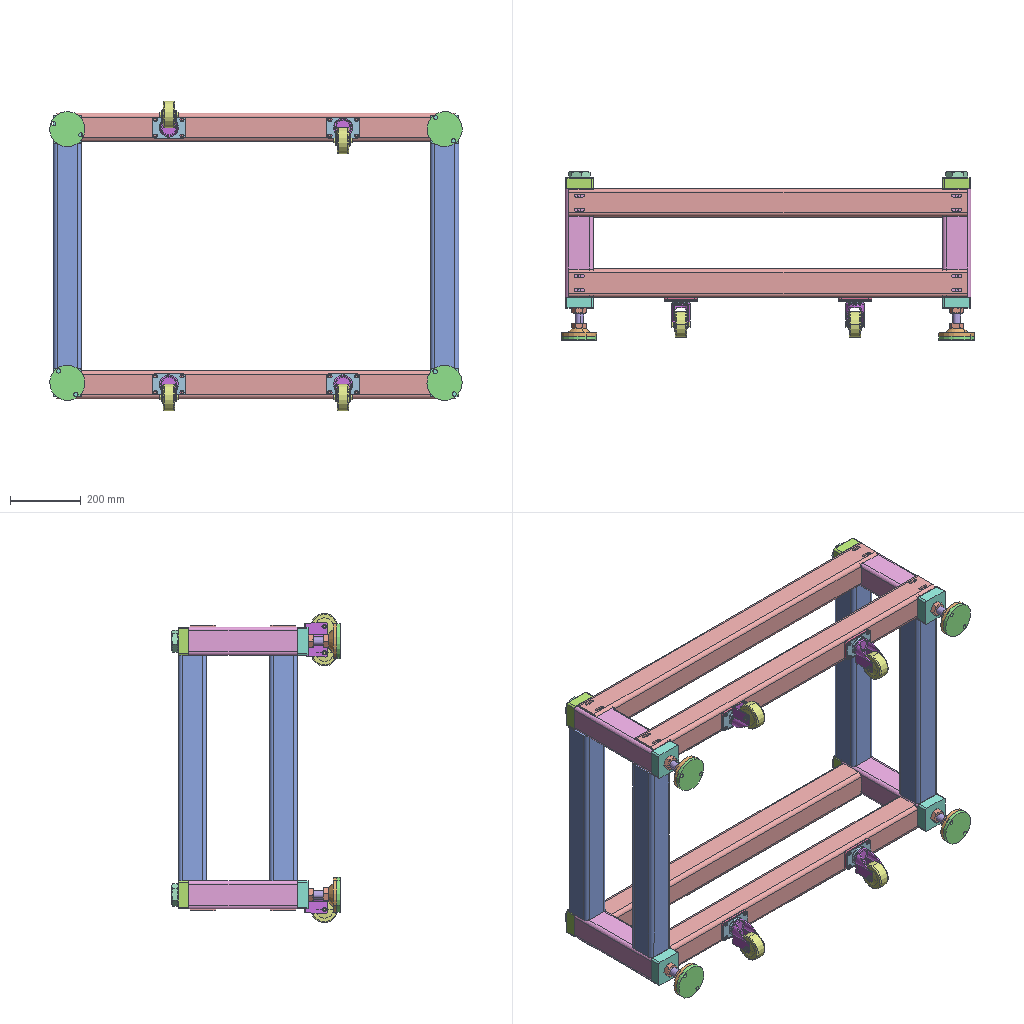Assembly | SolidWorks | 10 different items | 44 placed | box 1168 x 477 x 876 mm
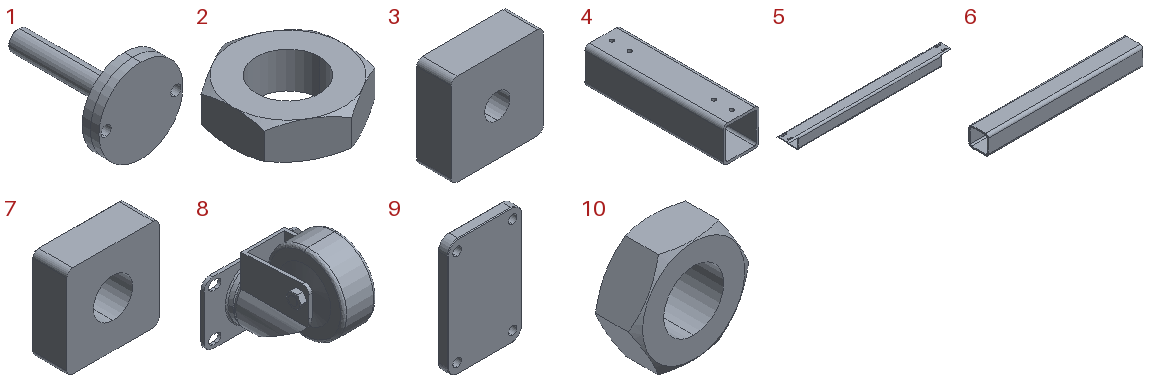Parts list (item | quantity | size | volume | features):
1 | x4 | 100 x 146 x 100 mm | 232661 mm3 | features BaseBody 3
2 | x4 | 55 x 63.509 x 18 mm | 32614 mm3 | features BaseBody 1
3 | x4 | 80 x 30 x 80 mm | 179952 mm3 | features Extrusion 1, Fillet 1, HoleWzd 1
4 | x4 | 80 x 307.64 x 80 mm | 500055 mm3 | features HoleWzd 3, Fillet 2, Extrusion 1, ICE 1
5 | x4 | 1128 x 80 x 80 mm | 1646266 mm3 | features ICE 3, Extrusion 1
6 | x4 | 638 x 80 x 80 mm | 1029649 mm3 | features Extrusion 1
7 | x4 | 80 x 30 x 80 mm | 164080 mm3 | features Chamfer 1, Extrusion 1, Fillet 1, HoleWzd 1
8 | x4 | 95 x 106 x 104.5 mm | 205443 mm3 | features ICE 4, BaseBody 2, Fillet 2, Extrusion 1, Revolution 1
9 | x4 | 60 x 8 x 95 mm | 43868 mm3 | features Chamfer 1, Extrusion 1, Fillet 1, HoleWzd 1
10 | x8 | 41.569 x 15 x 36.009 mm | 11607 mm3 | features Extrusion 1, RevCut 1
Mates (type | each side: item.copy, entity, surface, feature):
Coincident | 5.1 face plane Boss-Extrude1 | 4.1 face plane Boss-Extrude1 | 2 times
Coincident | 7.1 face plane Boss-Extrude1 | 4.1 face plane Boss-Extrude1 | 3 times
Coincident | 5.1 face plane Boss-Extrude1 | 4.2 face plane Boss-Extrude1 | 3 times
Coincident | 4.2 face plane Boss-Extrude1 | 7.2 face plane Boss-Extrude1 | 3 times
Coincident | 6.1 face plane Boss-Extrude1 | 7.2 face plane Boss-Extrude1 | 3 times
Coincident | 4.1 face plane Boss-Extrude1 | 5.1 face plane Boss-Extrude1
Coincident | 6.1 face plane Boss-Extrude1 | 7.3 face plane Boss-Extrude1 | 3 times
Coincident | 4.3 face plane Boss-Extrude1 | 7.3 face plane Boss-Extrude1 | 2 times
Coincident | 6.1 face plane Boss-Extrude1 | 4.3 face plane Boss-Extrude1
Coincident | 6.2 face plane Boss-Extrude1 | 4.1 face plane Boss-Extrude1 | 2 times
Coincident | 6.2 edge | 7.1 face plane Boss-Extrude1
Coincident | 4.4 face plane Boss-Extrude1 | 7.4 face plane Boss-Extrude1 | 2 times
Coincident | 4.4 edge | 7.4 face plane Boss-Extrude1
Coincident | 6.2 face plane Boss-Extrude1 | 7.4 face plane Boss-Extrude1 | 2 times
Coincident | 6.2 face plane Boss-Extrude1 | 4.4 face plane Boss-Extrude1
Coincident | 5.2 face plane Boss-Extrude1 | 4.4 face plane Boss-Extrude1
Coincident | 5.2 face plane Boss-Extrude1 | 7.4 edge
Coincident | 5.2 edge | 4.4 edge
Coincident | 4.4 face plane Boss-Extrude1 | 5.3 face plane Boss-Extrude1
Coincident | 4.4 edge | 5.3 edge
Coincident | 4.2 face plane Boss-Extrude1 | 5.4 face plane Boss-Extrude1
Coincident | 4.2 edge | 5.4 edge
Coincident | 4.1 face plane Boss-Extrude1 | 6.3 face plane Boss-Extrude1
Coincident | 4.4 edge | 6.3 edge
Coincident | 4.2 face plane Boss-Extrude1 | 6.4 face plane Boss-Extrude1
Coincident | 4.3 edge | 6.4 edge
Coincident | 4.3 face plane Boss-Extrude1 | 6.4 face plane Boss-Extrude1
Coincident | 4.1 face plane Boss-Extrude1 | 3.1 face plane Boss-Extrude1 | 3 times
Coincident | 4.4 face plane Boss-Extrude1 | 3.2 face plane Boss-Extrude1 | 3 times
Coincident | 4.2 face plane Boss-Extrude1 | 3.3 face plane Boss-Extrude1 | 3 times
Coincident | 4.3 face plane Boss-Extrude1 | 3.4 face plane Boss-Extrude1 | 3 times
Concentric | 3.1 edge | 1.1 edge
Concentric | 3.2 edge | 1.2 edge
Concentric | 3.3 edge | 1.3 edge
Concentric | 3.4 edge | 1.4 edge
Coincident | 9.1 face plane Boss-Extrude1 | 8.1 face plane Boss-Extrude1
Coincident | 9.2 face plane Boss-Extrude1 | 8.2 face plane Boss-Extrude1
Coincident | 9.3 face plane Boss-Extrude1 | 8.3 face plane Boss-Extrude1
Coincident | 9.4 face plane Boss-Extrude1 | 8.4 face plane Boss-Extrude1
Concentric | 9.2 edge | 8.2 edge
Concentric | 9.2 face cylinder Ø6.8 (6.8) Diameter Hole1 | 8.2 edge
Coincident | 5.4 face plane Boss-Extrude1 | 9.2 face plane Boss-Extrude1
Coincident | 5.4 edge | 3.1 edge
Coincident | 5.4 edge | 8.2 face plane Boss-Extrude1
Concentric | 9.3 edge | 8.3 edge | 2 times
Coincident | 5.4 face plane Boss-Extrude1 | 9.3 face plane Boss-Extrude1
Coincident | 5.4 edge | 9.3 face plane Boss-Extrude1
Concentric | 9.1 edge | 8.1 edge
Concentric | 9.1 edge | 8.1 face cylinder Cut-Extrude4
Concentric | 9.4 edge | 8.4 edge
Concentric | 9.4 face cylinder Ø6.8 (6.8) Diameter Hole1 | 8.4 edge
Coincident | 5.3 face plane Boss-Extrude1 | 9.4 face plane Boss-Extrude1
Coincident | 5.3 face plane Boss-Extrude1 | 9.1 face plane Boss-Extrude1
Coincident | 5.3 edge | 3.2 edge
Coincident | 5.3 edge | 9.1 face plane Boss-Extrude1
Coincident | 5.3 edge | 9.4 face plane Boss-Extrude1
Concentric | 7.3 edge | 2.1 edge
Concentric | 7.2 edge | 2.2 edge
Concentric | 7.1 edge | 2.3 edge
Concentric | 7.4 edge | 2.4 edge
Coincident | 7.2 face plane Boss-Extrude1 | 2.2 face plane Input1
Coincident | 7.3 face plane Boss-Extrude1 | 2.1 face plane Input1
Coincident | 7.4 face plane Boss-Extrude1 | 2.4 face plane Input1
Coincident | 7.1 face plane Boss-Extrude1 | 2.3 face plane Input1
DistanceDim | 1.1 face plane Input5 | 3.1 face plane Boss-Extrude1
DistanceDim | 3.2 face plane Boss-Extrude1 | 1.2 face plane Input5
Coincident | 1.1 face plane Input5 | 1.3 face plane Input5
Coincident | 1.4 face plane Input5 | 1.3 face plane Input5
DistanceDim | 9.3 face plane Boss-Extrude1 | 3.3 face plane Boss-Extrude1
DistanceDim | 9.2 face plane Boss-Extrude1 | 3.1 face plane Boss-Extrude1
Coincident | 9.4 face plane Boss-Extrude1 | 9.2 face plane Boss-Extrude1
Coincident | 9.3 face plane Boss-Extrude1 | 9.1 face plane Boss-Extrude1
Concentric | 1.2 face cylinder Input4 | 10.1 edge
Concentric | 1.2 face cylinder Input4 | 10.2 edge
Coincident | 3.2 face plane Boss-Extrude1 | 10.1 face plane Boss-Extrude1
Coincident | 1.2 face plane Input1 | 10.2 face plane Boss-Extrude1
Concentric | 1.1 face cylinder Input4 | 10.3 face cylinder Boss-Extrude1
Concentric | 1.1 face cylinder Input4 | 10.4 face cylinder Boss-Extrude1
Coincident | 3.1 face plane Boss-Extrude1 | 10.3 face plane Boss-Extrude1
Coincident | 1.1 face plane Input1 | 10.4 face plane Boss-Extrude1
Concentric | 1.3 face cylinder Input4 | 10.5 face cylinder Boss-Extrude1
Concentric | 1.3 face cylinder Input4 | 10.6 edge
Coincident | 3.3 face plane Boss-Extrude1 | 10.6 face plane Boss-Extrude1
Coincident | 1.3 face plane Input1 | 10.5 face plane Boss-Extrude1
Concentric | 1.4 face cylinder Input4 | 10.7 edge
Concentric | 1.4 face cylinder Input4 | 10.8 edge
Coincident | 3.4 face plane Boss-Extrude1 | 10.8 face plane Boss-Extrude1
Coincident | 1.4 face plane Input1 | 10.7 face plane Boss-Extrude1